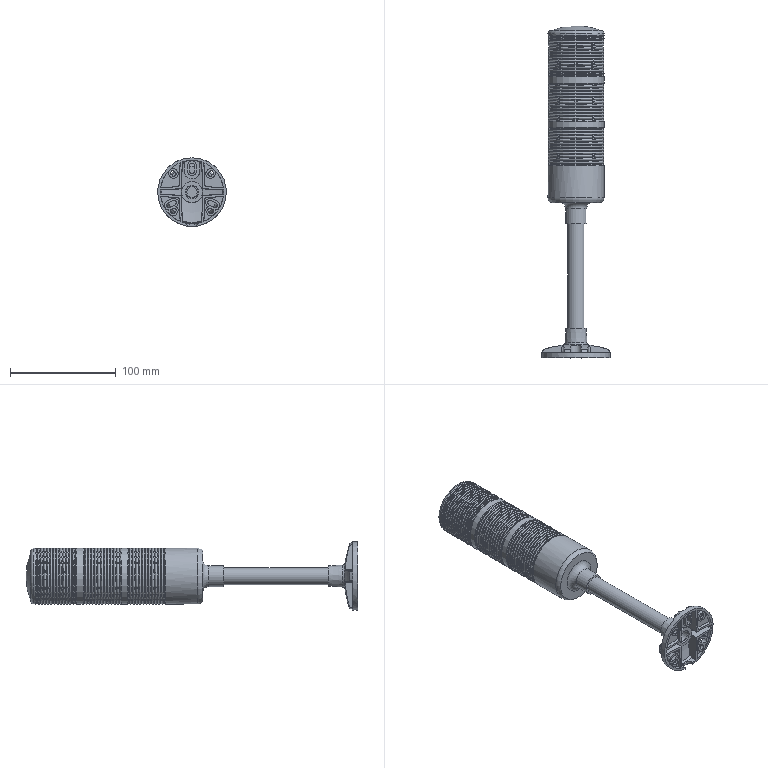Part | STEP file | E-MSM320RYG-C | 1 solid | 387 faces | box 65 x 314 x 64.82 mm | volume 382471 mm3 | torus 125 | cone 112 | plane 80 | cylinder 67 | sphere 2 | spline 1 | commonest cylinder face diameters 51.1 x37 4.5 x14 53 x6 5 x2 8.5 x2 10 x1